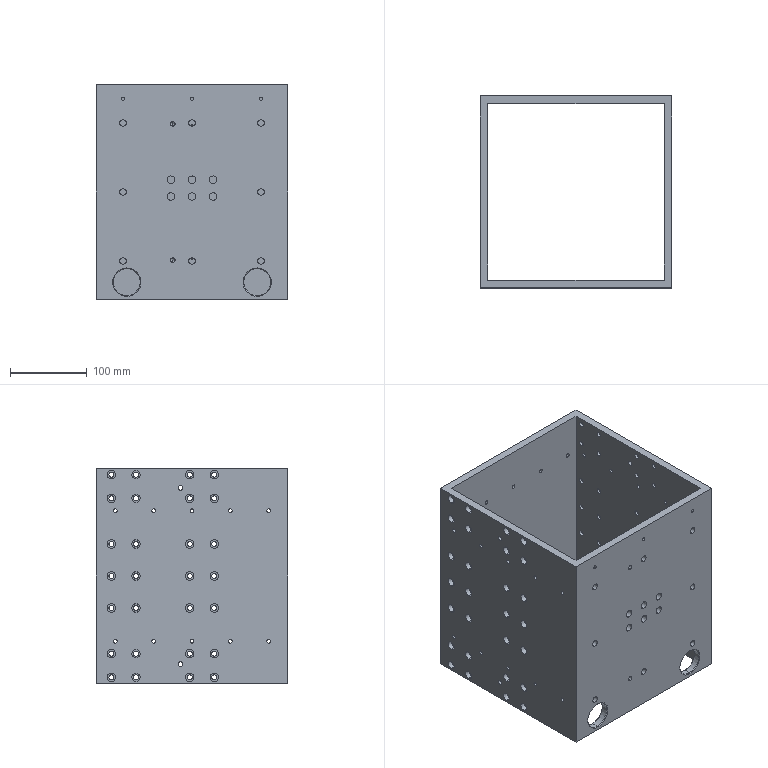Part | SolidWorks | features HoleWzd 8, Chamfer 1, Cut 1, Extrusion 1, MirrorPattern 1 | 1 solid | 412 faces | box 250 x 250 x 280 mm | volume 2610401 mm3 | cylinder 334 | plane 66 | cone 12 | commonest cylinder face diameters 6.6 x112 11 x112 5 x60 8.5 x16 6 x12 10 x12